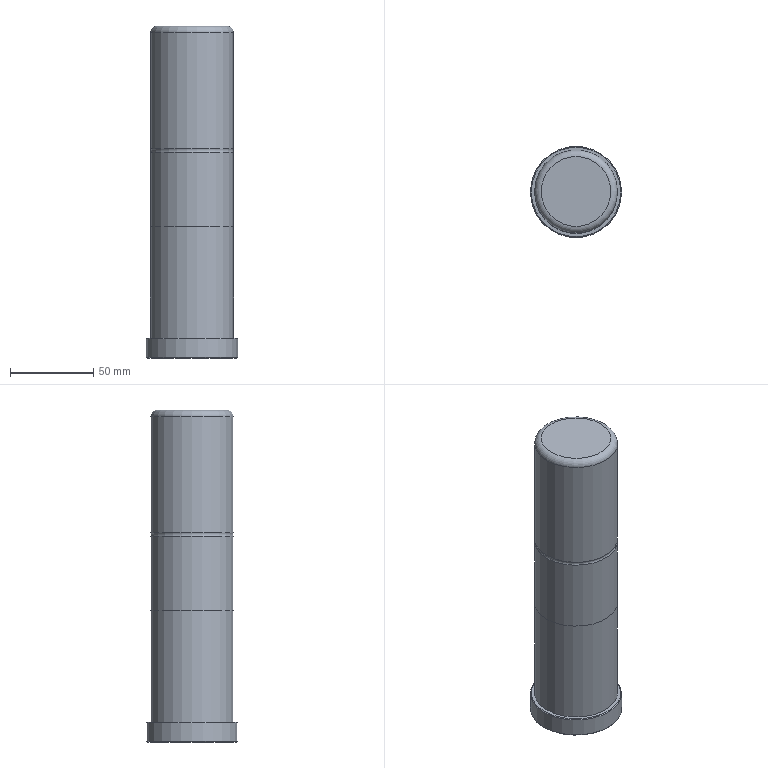Part | NX | features 模具.stp<1>[39] 2 | 1 solid | 12 faces | box 55 x 55 x 200 mm | volume 396989 mm3 | cylinder 4 | plane 4 | torus 2 | cone 2 | commonest cylinder face diameters 49.997 x2 50 x1 55 x1
STEP:
#1=CARTESIAN_POINT('',(271.998,-295.,95.5));
#2=VERTEX_POINT('',#1);
#3=CARTESIAN_POINT('',(247.,-295.,95.5));
#4=DIRECTION('',(0.,0.,-1.));
#5=DIRECTION('',(1.,0.,0.));
#6=AXIS2_PLACEMENT_3D('',#3,#4,#5);
#7=CIRCLE('',#6,24.998);
#8=EDGE_CURVE('',#2,#2,#7,.T.);
#9=ORIENTED_EDGE('',*,*,#8,.T.);
#10=EDGE_LOOP('',(#9));
#11=FACE_BOUND('',#10,.T.);
#12=CARTESIAN_POINT('',(222.001,-295.,25.551));
#13=VERTEX_POINT('',#12);
#14=CARTESIAN_POINT('',(247.,-295.,25.551));
#15=DIRECTION('',(0.,0.,-1.));
#16=DIRECTION('',(-1.,0.,0.));
#17=AXIS2_PLACEMENT_3D('',#14,#15,#16);
#18=CIRCLE('',#17,24.998);
#19=EDGE_CURVE('',#13,#13,#18,.T.);
#20=ORIENTED_EDGE('',*,*,#19,.F.);
#21=EDGE_LOOP('',(#20));
#22=FACE_BOUND('',#21,.T.);
#23=CARTESIAN_POINT('',(247.,-295.,-100.5));
#24=DIRECTION('',(0.,0.,1.));
#25=DIRECTION('',(1.,0.,0.));
#26=AXIS2_PLACEMENT_3D('',#23,#24,#25);
#27=CYLINDRICAL_SURFACE('',#26,24.998);
#28=ADVANCED_FACE('',(#11,#22),#27,.T.);
#29=ORIENTED_EDGE('',*,*,#8,.F.);
#30=EDGE_LOOP('',(#29));
#31=FACE_BOUND('',#30,.T.);
#32=CARTESIAN_POINT('',(267.998,-295.,99.5));
#33=VERTEX_POINT('',#32);
#34=CARTESIAN_POINT('',(247.,-295.,99.5));
#35=DIRECTION('',(0.,0.,1.));
#36=DIRECTION('',(1.,0.,0.));
#37=AXIS2_PLACEMENT_3D('',#34,#35,#36);
#38=CIRCLE('',#37,20.998);
#39=EDGE_CURVE('',#33,#33,#38,.T.);
#40=ORIENTED_EDGE('',*,*,#39,.F.);
#41=EDGE_LOOP('',(#40));
#42=FACE_BOUND('',#41,.T.);
#43=CARTESIAN_POINT('',(247.,-295.,95.5));
#44=DIRECTION('',(0.,0.,1.));
#45=DIRECTION('',(1.,0.,0.));
#46=AXIS2_PLACEMENT_3D('',#43,#44,#45);
#47=TOROIDAL_SURFACE('',#46,20.998,4.);
#48=ADVANCED_FACE('',(#31,#42),#47,.T.);
#49=ORIENTED_EDGE('',*,*,#39,.T.);
#50=EDGE_LOOP('',(#49));
#51=FACE_BOUND('',#50,.T.);
#52=CARTESIAN_POINT('',(247.,-295.,99.5));
#53=DIRECTION('',(0.,0.,1.));
#54=DIRECTION('',(1.,0.,0.));
#55=AXIS2_PLACEMENT_3D('',#52,#53,#54);
#56=PLANE('',#55);
#57=ADVANCED_FACE('',(#51),#56,.T.);
#58=CARTESIAN_POINT('',(271.998,-295.,23.449));
#59=VERTEX_POINT('',#58);
#60=CARTESIAN_POINT('',(247.,-295.,23.449));
#61=DIRECTION('',(0.,0.,1.));
#62=DIRECTION('',(1.,0.,0.));
#63=AXIS2_PLACEMENT_3D('',#60,#61,#62);
#64=CIRCLE('',#63,24.998);
#65=EDGE_CURVE('',#59,#59,#64,.T.);
#66=ORIENTED_EDGE('',*,*,#65,.T.);
#67=EDGE_LOOP('',(#66));
#68=FACE_BOUND('',#67,.T.);
#69=ORIENTED_EDGE('',*,*,#19,.T.);
#70=EDGE_LOOP('',(#69));
#71=FACE_BOUND('',#70,.T.);
#72=CARTESIAN_POINT('',(247.,-295.,24.5));
#73=DIRECTION('',(0.,0.,1.));
#74=DIRECTION('',(1.,0.,0.));
#75=AXIS2_PLACEMENT_3D('',#72,#73,#74);
#76=TOROIDAL_SURFACE('',#75,26.7,2.);
#77=ADVANCED_FACE('',(#68,#71),#76,.F.);
#78=CARTESIAN_POINT('',(271.998,-295.,-21.5));
#79=VERTEX_POINT('',#78);
#80=CARTESIAN_POINT('',(247.,-295.,-21.5));
#81=DIRECTION('',(0.,0.,1.));
#82=DIRECTION('',(1.,0.,0.));
#83=AXIS2_PLACEMENT_3D('',#80,#81,#82);
#84=CIRCLE('',#83,24.998);
#85=EDGE_CURVE('',#79,#79,#84,.T.);
#86=ORIENTED_EDGE('',*,*,#85,.T.);
#87=EDGE_LOOP('',(#86));
#88=FACE_BOUND('',#87,.T.);
#89=ORIENTED_EDGE('',*,*,#65,.F.);
#90=EDGE_LOOP('',(#89));
#91=FACE_BOUND('',#90,.T.);
#92=CARTESIAN_POINT('',(247.,-295.,-100.5));
#93=DIRECTION('',(0.,0.,1.));
#94=DIRECTION('',(1.,0.,0.));
#95=AXIS2_PLACEMENT_3D('',#92,#93,#94);
#96=CYLINDRICAL_SURFACE('',#95,24.998);
#97=ADVANCED_FACE('',(#88,#91),#96,.T.);
#98=CARTESIAN_POINT('',(272.,-295.,-21.5));
#99=VERTEX_POINT('',#98);
#100=CARTESIAN_POINT('',(247.,-295.,-21.5));
#101=DIRECTION('',(0.,0.,-1.));
#102=DIRECTION('',(1.,0.,0.));
#103=AXIS2_PLACEMENT_3D('',#100,#101,#102);
#104=CIRCLE('',#103,25.);
#105=EDGE_CURVE('',#99,#99,#104,.T.);
#106=ORIENTED_EDGE('',*,*,#105,.T.);
#107=EDGE_LOOP('',(#106));
#108=FACE_BOUND('',#107,.T.);
#109=CARTESIAN_POINT('',(272.,-295.,-88.5));
#110=VERTEX_POINT('',#109);
#111=CARTESIAN_POINT('',(247.,-295.,-88.5));
#112=DIRECTION('',(0.,0.,1.));
#113=DIRECTION('',(1.,0.,0.));
#114=AXIS2_PLACEMENT_3D('',#111,#112,#113);
#115=CIRCLE('',#114,25.);
#116=EDGE_CURVE('',#110,#110,#115,.T.);
#117=ORIENTED_EDGE('',*,*,#116,.T.);
#118=EDGE_LOOP('',(#117));
#119=FACE_BOUND('',#118,.T.);
#120=CARTESIAN_POINT('',(247.,-295.,-100.5));
#121=DIRECTION('',(0.,0.,1.));
#122=DIRECTION('',(1.,0.,0.));
#123=AXIS2_PLACEMENT_3D('',#120,#121,#122);
#124=CYLINDRICAL_SURFACE('',#123,25.);
#125=ADVANCED_FACE('',(#108,#119),#124,.T.);
#126=ORIENTED_EDGE('',*,*,#105,.F.);
#127=EDGE_LOOP('',(#126));
#128=FACE_BOUND('',#127,.T.);
#129=ORIENTED_EDGE('',*,*,#85,.F.);
#130=EDGE_LOOP('',(#129));
#131=FACE_BOUND('',#130,.T.);
#132=CARTESIAN_POINT('',(247.,-295.,-21.5));
#133=DIRECTION('',(0.,0.,1.));
#134=DIRECTION('',(1.,0.,0.));
#135=AXIS2_PLACEMENT_3D('',#132,#133,#134);
#136=PLANE('',#135);
#137=ADVANCED_FACE('',(#128,#131),#136,.T.);
#138=CARTESIAN_POINT('',(274.5,-295.,-89.));
#139=VERTEX_POINT('',#138);
#140=CARTESIAN_POINT('',(247.,-295.,-89.));
#141=DIRECTION('',(0.,0.,-1.));
#142=DIRECTION('',(1.,0.,0.));
#143=AXIS2_PLACEMENT_3D('',#140,#141,#142);
#144=CIRCLE('',#143,27.5);
#145=EDGE_CURVE('',#139,#139,#144,.T.);
#146=ORIENTED_EDGE('',*,*,#145,.F.);
#147=EDGE_LOOP('',(#146));
#148=FACE_BOUND('',#147,.T.);
#149=CARTESIAN_POINT('',(274.,-295.,-88.5));
#150=VERTEX_POINT('',#149);
#151=CARTESIAN_POINT('',(247.,-295.,-88.5));
#152=DIRECTION('',(0.,0.,1.));
#153=DIRECTION('',(1.,0.,0.));
#154=AXIS2_PLACEMENT_3D('',#151,#152,#153);
#155=CIRCLE('',#154,27.);
#156=EDGE_CURVE('',#150,#150,#155,.T.);
#157=ORIENTED_EDGE('',*,*,#156,.F.);
#158=EDGE_LOOP('',(#157));
#159=FACE_BOUND('',#158,.T.);
#160=CARTESIAN_POINT('',(247.,-295.,-89.));
#161=DIRECTION('',(0.,0.,-1.));
#162=DIRECTION('',(-1.,0.,0.));
#163=AXIS2_PLACEMENT_3D('',#160,#161,#162);
#164=CONICAL_SURFACE('',#163,27.5,0.7854);
#165=ADVANCED_FACE('',(#148,#159),#164,.T.);
#166=CARTESIAN_POINT('',(219.5,-295.,-100.));
#167=VERTEX_POINT('',#166);
#168=CARTESIAN_POINT('',(247.,-295.,-100.));
#169=DIRECTION('',(0.,0.,1.));
#170=DIRECTION('',(-1.,0.,0.));
#171=AXIS2_PLACEMENT_3D('',#168,#169,#170);
#172=CIRCLE('',#171,27.5);
#173=EDGE_CURVE('',#167,#167,#172,.T.);
#174=ORIENTED_EDGE('',*,*,#173,.F.);
#175=EDGE_LOOP('',(#174));
#176=FACE_BOUND('',#175,.T.);
#177=CARTESIAN_POINT('',(220.,-295.,-100.5));
#178=VERTEX_POINT('',#177);
#179=CARTESIAN_POINT('',(247.,-295.,-100.5));
#180=DIRECTION('',(0.,0.,-1.));
#181=DIRECTION('',(-1.,0.,0.));
#182=AXIS2_PLACEMENT_3D('',#179,#180,#181);
#183=CIRCLE('',#182,27.);
#184=EDGE_CURVE('',#178,#178,#183,.T.);
#185=ORIENTED_EDGE('',*,*,#184,.F.);
#186=EDGE_LOOP('',(#185));
#187=FACE_BOUND('',#186,.T.);
#188=CARTESIAN_POINT('',(247.,-295.,-100.));
#189=DIRECTION('',(0.,0.,1.));
#190=DIRECTION('',(1.,0.,0.));
#191=AXIS2_PLACEMENT_3D('',#188,#189,#190);
#192=CONICAL_SURFACE('',#191,27.5,0.7854);
#193=ADVANCED_FACE('',(#176,#187),#192,.T.);
#194=ORIENTED_EDGE('',*,*,#145,.T.);
#195=EDGE_LOOP('',(#194));
#196=FACE_BOUND('',#195,.T.);
#197=ORIENTED_EDGE('',*,*,#173,.T.);
#198=EDGE_LOOP('',(#197));
#199=FACE_BOUND('',#198,.T.);
#200=CARTESIAN_POINT('',(247.,-295.,-100.5));
#201=DIRECTION('',(0.,0.,1.));
#202=DIRECTION('',(1.,0.,0.));
#203=AXIS2_PLACEMENT_3D('',#200,#201,#202);
#204=CYLINDRICAL_SURFACE('',#203,27.5);
#205=ADVANCED_FACE('',(#196,#199),#204,.T.);
#206=ORIENTED_EDGE('',*,*,#184,.T.);
#207=EDGE_LOOP('',(#206));
#208=FACE_BOUND('',#207,.T.);
#209=CARTESIAN_POINT('',(247.,-295.,-100.5));
#210=DIRECTION('',(0.,0.,-1.));
#211=DIRECTION('',(0.,-1.,0.));
#212=AXIS2_PLACEMENT_3D('',#209,#210,#211);
#213=PLANE('',#212);
#214=ADVANCED_FACE('',(#208),#213,.T.);
#215=ORIENTED_EDGE('',*,*,#156,.T.);
#216=EDGE_LOOP('',(#215));
#217=FACE_BOUND('',#216,.T.);
#218=ORIENTED_EDGE('',*,*,#116,.F.);
#219=EDGE_LOOP('',(#218));
#220=FACE_BOUND('',#219,.T.);
#221=CARTESIAN_POINT('',(247.,-295.,-88.5));
#222=DIRECTION('',(0.,0.,1.));
#223=DIRECTION('',(1.,0.,0.));
#224=AXIS2_PLACEMENT_3D('',#221,#222,#223);
#225=PLANE('',#224);
#226=ADVANCED_FACE('',(#217,#220),#225,.T.);
#227=CLOSED_SHELL('',(#28,#48,#57,#77,#97,#125,#137,#165,#193,#205,#214,#226));
#228=MANIFOLD_SOLID_BREP('',#227);
#229=(LENGTH_UNIT()NAMED_UNIT(*)SI_UNIT(.MILLI.,.METRE.));
#230=UNCERTAINTY_MEASURE_WITH_UNIT(LENGTH_MEASURE(0.00001),#229,'','');
#231=(NAMED_UNIT(*)PLANE_ANGLE_UNIT()SI_UNIT($,.RADIAN.));
#232=(NAMED_UNIT(*)SI_UNIT($,.STERADIAN.)SOLID_ANGLE_UNIT());
#233=(GEOMETRIC_REPRESENTATION_CONTEXT(3)GLOBAL_UNCERTAINTY_ASSIGNED_CONTEXT((#230))GLOBAL_UNIT_ASSIGNED_CONTEXT((#229,#231,#232))REPRESENTATION_CONTEXT('',''));
#234=ADVANCED_BREP_SHAPE_REPRESENTATION('',(#228),#233);